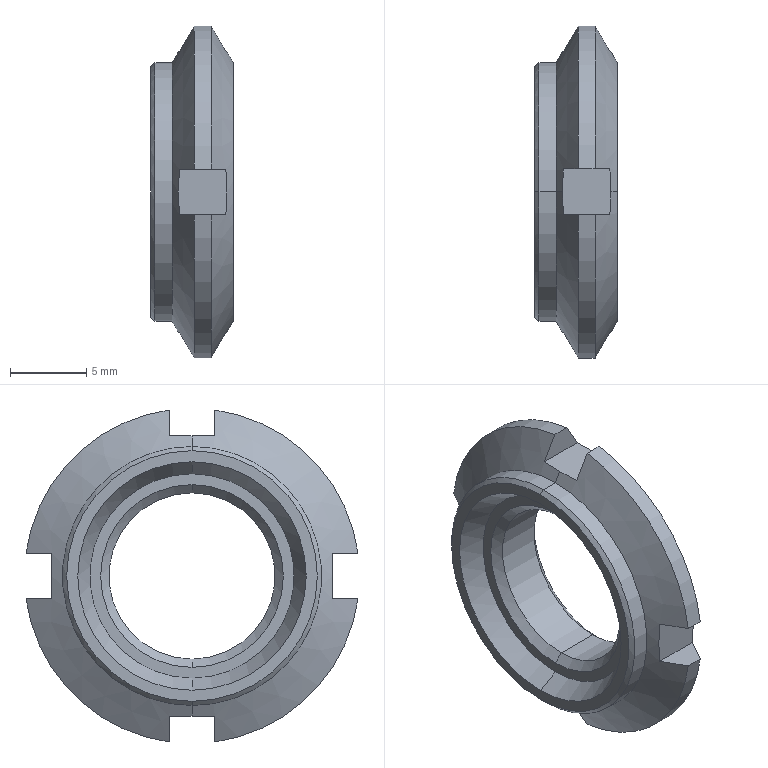Part | STEP file | funt12_2_03 | 1 solid | 35 faces | box 5.4 x 21.794 x 21.794 mm | volume 953.545 mm3 | plane 15 | cone 12 | cylinder 8 | commonest cylinder face diameters 22 x4 10.917 x2 17 x2